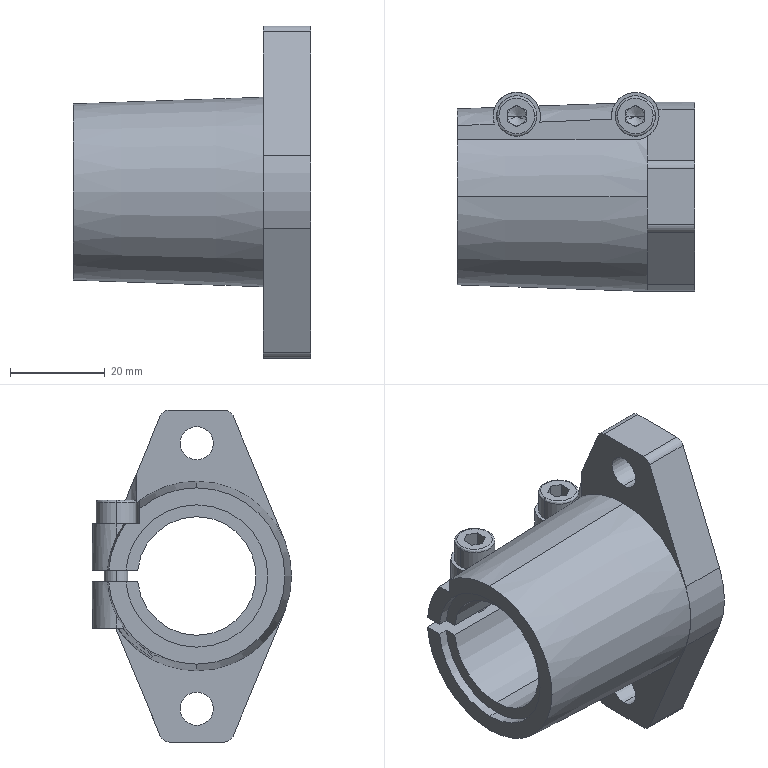Part | SolidWorks | features BaseBody 3 | 3 solids | 137 faces | box 50 x 42 x 70 mm | volume 41488 mm3 | plane 47 | cylinder 45 | cone 33 | spline 12 | commonest cylinder face diameters 10 x10 4.134 x8 5 x5 4 x4 7 x4 8.5 x4